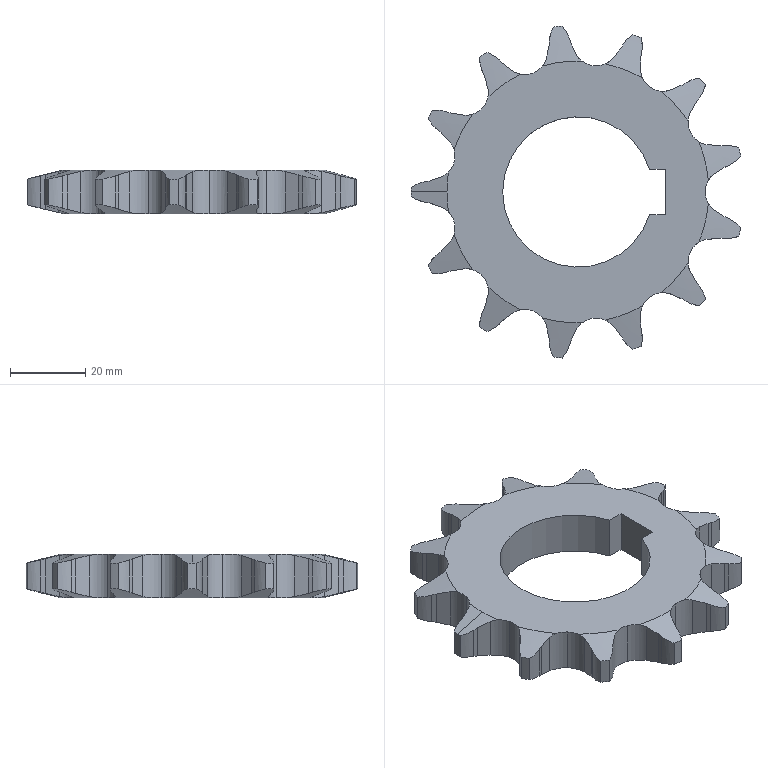Part | SolidWorks | features BaseBody 1 | 1 solid | 150 faces | box 87.7 x 88.328 x 11.659 mm | volume 36019 mm3 | cylinder 92 | plane 31 | cone 27 | commonest cylinder face diameters 12.048 x26 20.1 x26 31.109 x26 88.719 x13 40 x1